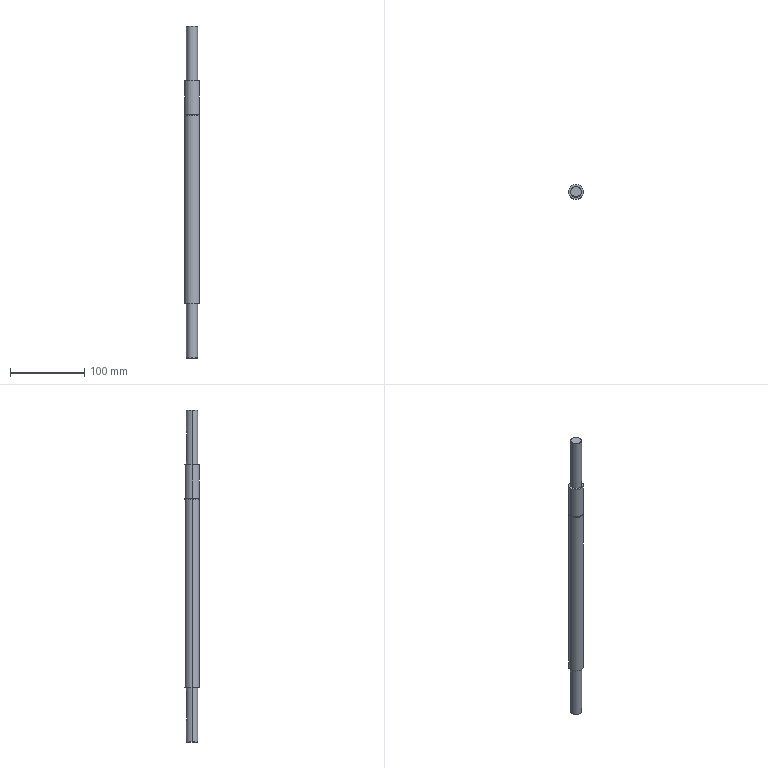Part | SolidWorks | features ICE 5, Chamfer 1, Cut 1, Extrusion 1 | 1 solid | 32 faces | box 20 x 20 x 448 mm | volume 119242 mm3 | cylinder 16 | plane 12 | cone 4 | commonest cylinder face diameters 5 x6 15 x4 20 x4 19 x2
STEP:
#1=CARTESIAN_POINT('',(10.,0.,300.));
#2=VERTEX_POINT('',#1);
#3=CARTESIAN_POINT('',(-10.,0.,300.));
#4=VERTEX_POINT('',#3);
#5=CARTESIAN_POINT('',(0.,0.,300.));
#6=DIRECTION('',(0.,0.,1.));
#7=DIRECTION('',(1.,0.,0.));
#8=AXIS2_PLACEMENT_3D('',#5,#6,#7);
#9=CIRCLE('',#8,10.);
#10=EDGE_CURVE('',#2,#4,#9,.T.);
#11=ORIENTED_EDGE('',*,*,#10,.F.);
#12=CARTESIAN_POINT('',(10.,0.,255.));
#13=VERTEX_POINT('',#12);
#14=CARTESIAN_POINT('',(10.,0.,300.));
#15=DIRECTION('',(0.,0.,-1.));
#16=VECTOR('',#15,1000.);
#17=LINE('',#14,#16);
#18=EDGE_CURVE('',#2,#13,#17,.T.);
#19=ORIENTED_EDGE('',*,*,#18,.T.);
#20=CARTESIAN_POINT('',(-10.,0.,255.));
#21=VERTEX_POINT('',#20);
#22=CARTESIAN_POINT('',(0.,0.,255.));
#23=DIRECTION('',(0.,0.,-1.));
#24=DIRECTION('',(0.,1.,0.));
#25=AXIS2_PLACEMENT_3D('',#22,#23,#24);
#26=CIRCLE('',#25,10.);
#27=EDGE_CURVE('',#21,#13,#26,.T.);
#28=ORIENTED_EDGE('',*,*,#27,.F.);
#29=CARTESIAN_POINT('',(-10.,0.,300.));
#30=DIRECTION('',(0.,0.,-1.));
#31=VECTOR('',#30,1000.);
#32=LINE('',#29,#31);
#33=EDGE_CURVE('',#4,#21,#32,.T.);
#34=ORIENTED_EDGE('',*,*,#33,.F.);
#35=EDGE_LOOP('',(#11,#19,#28,#34));
#36=FACE_OUTER_BOUND('',#35,.T.);
#37=CARTESIAN_POINT('',(0.,0.,300.));
#38=DIRECTION('',(0.,0.,-1.));
#39=DIRECTION('',(-1.,0.,0.));
#40=AXIS2_PLACEMENT_3D('',#37,#38,#39);
#41=CYLINDRICAL_SURFACE('',#40,10.);
#42=ADVANCED_FACE('',(#36),#41,.T.);
#43=CARTESIAN_POINT('',(2.5,7.071,343.));
#44=VERTEX_POINT('',#43);
#45=CARTESIAN_POINT('',(0.,7.5,345.5));
#46=VERTEX_POINT('',#45);
#47=CARTESIAN_POINT('',(2.5,7.071,343.));
#48=CARTESIAN_POINT('',(2.5,7.071,343.165));
#49=CARTESIAN_POINT('',(2.484,7.077,343.328));
#50=CARTESIAN_POINT('',(2.419,7.099,343.651));
#51=CARTESIAN_POINT('',(2.371,7.116,343.81));
#52=CARTESIAN_POINT('',(2.183,7.177,344.262));
#53=CARTESIAN_POINT('',(1.997,7.233,344.538));
#54=CARTESIAN_POINT('',(1.654,7.316,344.882));
#55=CARTESIAN_POINT('',(1.526,7.344,344.987));
#56=CARTESIAN_POINT('',(1.256,7.395,345.168));
#57=CARTESIAN_POINT('',(1.113,7.419,345.245));
#58=CARTESIAN_POINT('',(0.8106,7.458,345.371));
#59=CARTESIAN_POINT('',(0.6511,7.473,345.419));
#60=CARTESIAN_POINT('',(0.33,7.494,345.484));
#61=CARTESIAN_POINT('',(0.1664,7.5,345.5));
#62=CARTESIAN_POINT('',(0.,7.5,345.5));
#63=B_SPLINE_CURVE_WITH_KNOTS('',3,(#47,#48,#49,#50,#51,#52,#53,#54,#55,#56,#57,#58,#59,#60,#61,#62),.UNSPECIFIED.,.F.,.F.,(4,2,2,2,2,2,2,4),(0.01181,0.0123,0.01279,0.01378,0.01427,0.01476,0.01525,0.01574),.UNSPECIFIED.);
#64=EDGE_CURVE('',#44,#46,#63,.T.);
#65=ORIENTED_EDGE('',*,*,#64,.T.);
#66=CARTESIAN_POINT('',(-2.5,7.071,343.));
#67=VERTEX_POINT('',#66);
#68=CARTESIAN_POINT('',(0.,7.5,345.5));
#69=CARTESIAN_POINT('',(-0.1665,7.5,345.5));
#70=CARTESIAN_POINT('',(-0.33,7.494,345.484));
#71=CARTESIAN_POINT('',(-0.6513,7.473,345.419));
#72=CARTESIAN_POINT('',(-0.8108,7.458,345.371));
#73=CARTESIAN_POINT('',(-1.113,7.418,345.244));
#74=CARTESIAN_POINT('',(-1.256,7.395,345.167));
#75=CARTESIAN_POINT('',(-1.527,7.344,344.986));
#76=CARTESIAN_POINT('',(-1.655,7.316,344.881));
#77=CARTESIAN_POINT('',(-1.998,7.233,344.537));
#78=CARTESIAN_POINT('',(-2.183,7.176,344.26));
#79=CARTESIAN_POINT('',(-2.371,7.116,343.81));
#80=CARTESIAN_POINT('',(-2.419,7.099,343.651));
#81=CARTESIAN_POINT('',(-2.484,7.077,343.328));
#82=CARTESIAN_POINT('',(-2.5,7.071,343.164));
#83=CARTESIAN_POINT('',(-2.5,7.071,343.));
#84=B_SPLINE_CURVE_WITH_KNOTS('',3,(#68,#69,#70,#71,#72,#73,#74,#75,#76,#77,#78,#79,#80,#81,#82,#83),.UNSPECIFIED.,.F.,.F.,(4,2,2,2,2,2,2,4),(0.,0.0004922,0.0009844,0.001477,0.001969,0.002953,0.003445,0.003938),.UNSPECIFIED.);
#85=EDGE_CURVE('',#46,#67,#84,.T.);
#86=ORIENTED_EDGE('',*,*,#85,.T.);
#87=CARTESIAN_POINT('',(-2.5,7.071,308.));
#88=VERTEX_POINT('',#87);
#89=CARTESIAN_POINT('',(-2.5,7.071,374.));
#90=DIRECTION('',(0.,0.,-1.));
#91=VECTOR('',#90,1000.);
#92=LINE('',#89,#91);
#93=EDGE_CURVE('',#67,#88,#92,.T.);
#94=ORIENTED_EDGE('',*,*,#93,.T.);
#95=CARTESIAN_POINT('',(2.5,7.071,308.));
#96=VERTEX_POINT('',#95);
#97=CARTESIAN_POINT('',(-2.5,7.071,308.));
#98=CARTESIAN_POINT('',(-2.5,7.071,307.836));
#99=CARTESIAN_POINT('',(-2.483,7.077,307.669));
#100=CARTESIAN_POINT('',(-2.419,7.099,307.347));
#101=CARTESIAN_POINT('',(-2.371,7.116,307.191));
#102=CARTESIAN_POINT('',(-2.244,7.157,306.887));
#103=CARTESIAN_POINT('',(-2.167,7.181,306.743));
#104=CARTESIAN_POINT('',(-1.986,7.233,306.473));
#105=CARTESIAN_POINT('',(-1.882,7.261,306.346));
#106=CARTESIAN_POINT('',(-1.652,7.317,306.116));
#107=CARTESIAN_POINT('',(-1.527,7.344,306.014));
#108=CARTESIAN_POINT('',(-1.257,7.395,305.833));
#109=CARTESIAN_POINT('',(-1.11,7.419,305.754));
#110=CARTESIAN_POINT('',(-0.8093,7.458,305.629));
#111=CARTESIAN_POINT('',(-0.6533,7.473,305.581));
#112=CARTESIAN_POINT('',(-0.3296,7.495,305.516));
#113=CARTESIAN_POINT('',(-0.164,7.5,305.5));
#114=CARTESIAN_POINT('',(0.1639,7.5,305.5));
#115=CARTESIAN_POINT('',(0.329,7.495,305.516));
#116=CARTESIAN_POINT('',(0.6533,7.473,305.581));
#117=CARTESIAN_POINT('',(0.8096,7.458,305.629));
#118=CARTESIAN_POINT('',(1.111,7.419,305.755));
#119=CARTESIAN_POINT('',(1.257,7.395,305.833));
#120=CARTESIAN_POINT('',(1.527,7.344,306.014));
#121=CARTESIAN_POINT('',(1.653,7.317,306.117));
#122=CARTESIAN_POINT('',(1.999,7.233,306.463));
#123=CARTESIAN_POINT('',(2.182,7.177,306.736));
#124=CARTESIAN_POINT('',(2.371,7.116,307.192));
#125=CARTESIAN_POINT('',(2.419,7.099,307.348));
#126=CARTESIAN_POINT('',(2.483,7.077,307.669));
#127=CARTESIAN_POINT('',(2.5,7.071,307.835));
#128=CARTESIAN_POINT('',(2.5,7.071,308.));
#129=B_SPLINE_CURVE_WITH_KNOTS('',3,(#97,#98,#99,#100,#101,#102,#103,#104,#105,#106,#107,#108,#109,#110,#111,#112,#113,#114,#115,#116,#117,#118,#119,#120,#121,#122,#123,#124,#125,#126,#127,#128),.UNSPECIFIED.,.F.,.F.,(4,2,2,2,2,2,2,2,2,2,2,2,2,2,2,4),(0.003938,0.00443,0.004921,0.005413,0.005905,0.006397,0.006889,0.007381,0.007873,0.008365,0.008857,0.009349,0.00984,0.01082,0.01132,0.01181),.UNSPECIFIED.);
#130=EDGE_CURVE('',#88,#96,#129,.T.);
#131=ORIENTED_EDGE('',*,*,#130,.T.);
#132=CARTESIAN_POINT('',(2.5,7.071,374.));
#133=DIRECTION('',(0.,0.,1.));
#134=VECTOR('',#133,1000.);
#135=LINE('',#132,#134);
#136=EDGE_CURVE('',#96,#44,#135,.T.);
#137=ORIENTED_EDGE('',*,*,#136,.T.);
#138=EDGE_LOOP('',(#65,#86,#94,#131,#137));
#139=FACE_BOUND('',#138,.T.);
#140=CARTESIAN_POINT('',(-7.5,0.,373.5));
#141=VERTEX_POINT('',#140);
#142=CARTESIAN_POINT('',(7.5,0.,373.5));
#143=VERTEX_POINT('',#142);
#144=CARTESIAN_POINT('',(0.,0.,373.5));
#145=DIRECTION('',(0.,0.,-1.));
#146=DIRECTION('',(1.,0.,0.));
#147=AXIS2_PLACEMENT_3D('',#144,#145,#146);
#148=CIRCLE('',#147,7.5);
#149=EDGE_CURVE('',#141,#143,#148,.T.);
#150=ORIENTED_EDGE('',*,*,#149,.T.);
#151=CARTESIAN_POINT('',(7.5,0.,300.));
#152=VERTEX_POINT('',#151);
#153=CARTESIAN_POINT('',(7.5,0.,374.));
#154=DIRECTION('',(0.,0.,-1.));
#155=VECTOR('',#154,1000.);
#156=LINE('',#153,#155);
#157=EDGE_CURVE('',#143,#152,#156,.T.);
#158=ORIENTED_EDGE('',*,*,#157,.T.);
#159=CARTESIAN_POINT('',(-7.5,0.,300.));
#160=VERTEX_POINT('',#159);
#161=CARTESIAN_POINT('',(0.,0.,300.));
#162=DIRECTION('',(0.,0.,1.));
#163=DIRECTION('',(1.,0.,0.));
#164=AXIS2_PLACEMENT_3D('',#161,#162,#163);
#165=CIRCLE('',#164,7.5);
#166=EDGE_CURVE('',#152,#160,#165,.T.);
#167=ORIENTED_EDGE('',*,*,#166,.T.);
#168=CARTESIAN_POINT('',(-7.5,0.,374.));
#169=DIRECTION('',(0.,0.,-1.));
#170=VECTOR('',#169,1000.);
#171=LINE('',#168,#170);
#172=EDGE_CURVE('',#141,#160,#171,.T.);
#173=ORIENTED_EDGE('',*,*,#172,.F.);
#174=EDGE_LOOP('',(#150,#158,#167,#173));
#175=FACE_OUTER_BOUND('',#174,.T.);
#176=CARTESIAN_POINT('',(0.,0.,374.));
#177=DIRECTION('',(0.,0.,-1.));
#178=DIRECTION('',(-1.,0.,0.));
#179=AXIS2_PLACEMENT_3D('',#176,#177,#178);
#180=CYLINDRICAL_SURFACE('',#179,7.5);
#181=ADVANCED_FACE('',(#139,#175),#180,.T.);
#182=CARTESIAN_POINT('',(7.,0.,374.));
#183=VERTEX_POINT('',#182);
#184=CARTESIAN_POINT('',(-7.,0.,374.));
#185=VERTEX_POINT('',#184);
#186=CARTESIAN_POINT('',(0.,0.,374.));
#187=DIRECTION('',(0.,0.,1.));
#188=DIRECTION('',(1.,0.,0.));
#189=AXIS2_PLACEMENT_3D('',#186,#187,#188);
#190=CIRCLE('',#189,7.);
#191=EDGE_CURVE('',#183,#185,#190,.T.);
#192=ORIENTED_EDGE('',*,*,#191,.F.);
#193=CARTESIAN_POINT('',(7.,0.,374.));
#194=DIRECTION('',(0.7071,0.,-0.7071));
#195=VECTOR('',#194,1000.);
#196=LINE('',#193,#195);
#197=EDGE_CURVE('',#183,#143,#196,.T.);
#198=ORIENTED_EDGE('',*,*,#197,.T.);
#199=ORIENTED_EDGE('',*,*,#149,.F.);
#200=CARTESIAN_POINT('',(-7.,0.,374.));
#201=DIRECTION('',(-0.7071,0.,-0.7071));
#202=VECTOR('',#201,1000.);
#203=LINE('',#200,#202);
#204=EDGE_CURVE('',#185,#141,#203,.T.);
#205=ORIENTED_EDGE('',*,*,#204,.F.);
#206=EDGE_LOOP('',(#192,#198,#199,#205));
#207=FACE_OUTER_BOUND('',#206,.T.);
#208=CARTESIAN_POINT('',(0.,0.,374.));
#209=DIRECTION('',(0.,0.,-1.));
#210=DIRECTION('',(-1.,0.,0.));
#211=AXIS2_PLACEMENT_3D('',#208,#209,#210);
#212=CONICAL_SURFACE('',#211,7.,0.7854);
#213=ADVANCED_FACE('',(#207),#212,.T.);
#214=CARTESIAN_POINT('',(0.,4.5,345.5));
#215=VERTEX_POINT('',#214);
#216=CARTESIAN_POINT('',(2.5,4.5,343.));
#217=VERTEX_POINT('',#216);
#218=CARTESIAN_POINT('',(0.,4.5,343.));
#219=DIRECTION('',(0.,1.,0.));
#220=DIRECTION('',(0.,0.,1.));
#221=AXIS2_PLACEMENT_3D('',#218,#219,#220);
#222=CIRCLE('',#221,2.5);
#223=EDGE_CURVE('',#215,#217,#222,.T.);
#224=ORIENTED_EDGE('',*,*,#223,.F.);
#225=CARTESIAN_POINT('',(0.,4.5,345.5));
#226=DIRECTION('',(0.,1.,0.));
#227=VECTOR('',#226,1000.);
#228=LINE('',#225,#227);
#229=EDGE_CURVE('',#215,#46,#228,.T.);
#230=ORIENTED_EDGE('',*,*,#229,.T.);
#231=ORIENTED_EDGE('',*,*,#64,.F.);
#232=CARTESIAN_POINT('',(2.5,4.5,343.));
#233=DIRECTION('',(0.,1.,0.));
#234=VECTOR('',#233,1000.);
#235=LINE('',#232,#234);
#236=EDGE_CURVE('',#217,#44,#235,.T.);
#237=ORIENTED_EDGE('',*,*,#236,.F.);
#238=EDGE_LOOP('',(#224,#230,#231,#237));
#239=FACE_OUTER_BOUND('',#238,.T.);
#240=CARTESIAN_POINT('',(0.,4.5,343.));
#241=DIRECTION('',(0.,1.,0.));
#242=DIRECTION('',(0.,0.,1.));
#243=AXIS2_PLACEMENT_3D('',#240,#241,#242);
#244=CYLINDRICAL_SURFACE('',#243,2.5);
#245=ADVANCED_FACE('',(#239),#244,.F.);
#246=CARTESIAN_POINT('',(0.,9.5,253.9));
#247=VERTEX_POINT('',#246);
#248=CARTESIAN_POINT('',(0.,-9.5,253.9));
#249=VERTEX_POINT('',#248);
#250=CARTESIAN_POINT('',(0.,0.,253.9));
#251=DIRECTION('',(0.,0.,-1.));
#252=DIRECTION('',(0.,1.,0.));
#253=AXIS2_PLACEMENT_3D('',#250,#251,#252);
#254=CIRCLE('',#253,9.5);
#255=EDGE_CURVE('',#247,#249,#254,.T.);
#256=ORIENTED_EDGE('',*,*,#255,.F.);
#257=CARTESIAN_POINT('',(0.,9.5,255.));
#258=VERTEX_POINT('',#257);
#259=CARTESIAN_POINT('',(0.,9.5,253.9));
#260=DIRECTION('',(0.,0.,1.));
#261=VECTOR('',#260,1000.);
#262=LINE('',#259,#261);
#263=EDGE_CURVE('',#247,#258,#262,.T.);
#264=ORIENTED_EDGE('',*,*,#263,.T.);
#265=CARTESIAN_POINT('',(0.,-9.5,255.));
#266=VERTEX_POINT('',#265);
#267=CARTESIAN_POINT('',(0.,0.,255.));
#268=DIRECTION('',(0.,0.,-1.));
#269=DIRECTION('',(0.,1.,0.));
#270=AXIS2_PLACEMENT_3D('',#267,#268,#269);
#271=CIRCLE('',#270,9.5);
#272=EDGE_CURVE('',#258,#266,#271,.T.);
#273=ORIENTED_EDGE('',*,*,#272,.T.);
#274=CARTESIAN_POINT('',(0.,-9.5,253.9));
#275=DIRECTION('',(0.,0.,1.));
#276=VECTOR('',#275,1000.);
#277=LINE('',#274,#276);
#278=EDGE_CURVE('',#249,#266,#277,.T.);
#279=ORIENTED_EDGE('',*,*,#278,.F.);
#280=EDGE_LOOP('',(#256,#264,#273,#279));
#281=FACE_OUTER_BOUND('',#280,.T.);
#282=CARTESIAN_POINT('',(0.,0.,253.9));
#283=DIRECTION('',(0.,0.,1.));
#284=DIRECTION('',(0.,-1.,0.));
#285=AXIS2_PLACEMENT_3D('',#282,#283,#284);
#286=CYLINDRICAL_SURFACE('',#285,9.5);
#287=ADVANCED_FACE('',(#281),#286,.T.);
#288=CARTESIAN_POINT('',(-7.,0.,-74.));
#289=VERTEX_POINT('',#288);
#290=CARTESIAN_POINT('',(7.,0.,-74.));
#291=VERTEX_POINT('',#290);
#292=CARTESIAN_POINT('',(0.,0.,-74.));
#293=DIRECTION('',(0.,0.,-1.));
#294=DIRECTION('',(-1.,0.,0.));
#295=AXIS2_PLACEMENT_3D('',#292,#293,#294);
#296=CIRCLE('',#295,7.);
#297=EDGE_CURVE('',#289,#291,#296,.T.);
#298=ORIENTED_EDGE('',*,*,#297,.F.);
#299=CARTESIAN_POINT('',(-7.5,0.,-73.5));
#300=VERTEX_POINT('',#299);
#301=CARTESIAN_POINT('',(-7.,0.,-74.));
#302=DIRECTION('',(-0.7071,0.,0.7071));
#303=VECTOR('',#302,1000.);
#304=LINE('',#301,#303);
#305=EDGE_CURVE('',#289,#300,#304,.T.);
#306=ORIENTED_EDGE('',*,*,#305,.T.);
#307=CARTESIAN_POINT('',(7.5,0.,-73.5));
#308=VERTEX_POINT('',#307);
#309=CARTESIAN_POINT('',(0.,0.,-73.5));
#310=DIRECTION('',(0.,0.,1.));
#311=DIRECTION('',(-1.,0.,0.));
#312=AXIS2_PLACEMENT_3D('',#309,#310,#311);
#313=CIRCLE('',#312,7.5);
#314=EDGE_CURVE('',#308,#300,#313,.T.);
#315=ORIENTED_EDGE('',*,*,#314,.F.);
#316=CARTESIAN_POINT('',(7.,0.,-74.));
#317=DIRECTION('',(0.7071,0.,0.7071));
#318=VECTOR('',#317,1000.);
#319=LINE('',#316,#318);
#320=EDGE_CURVE('',#291,#308,#319,.T.);
#321=ORIENTED_EDGE('',*,*,#320,.F.);
#322=EDGE_LOOP('',(#298,#306,#315,#321));
#323=FACE_OUTER_BOUND('',#322,.T.);
#324=CARTESIAN_POINT('',(0.,0.,-74.));
#325=DIRECTION('',(0.,0.,1.));
#326=DIRECTION('',(1.,0.,0.));
#327=AXIS2_PLACEMENT_3D('',#324,#325,#326);
#328=CONICAL_SURFACE('',#327,7.,0.7854);
#329=ADVANCED_FACE('',(#323),#328,.T.);
#330=CARTESIAN_POINT('',(0.,4.5,-5.5));
#331=VERTEX_POINT('',#330);
#332=CARTESIAN_POINT('',(2.5,4.5,-8.));
#333=VERTEX_POINT('',#332);
#334=CARTESIAN_POINT('',(0.,4.5,-8.));
#335=DIRECTION('',(0.,1.,0.));
#336=DIRECTION('',(0.,0.,1.));
#337=AXIS2_PLACEMENT_3D('',#334,#335,#336);
#338=CIRCLE('',#337,2.5);
#339=EDGE_CURVE('',#331,#333,#338,.T.);
#340=ORIENTED_EDGE('',*,*,#339,.F.);
#341=CARTESIAN_POINT('',(0.,7.5,-5.5));
#342=VERTEX_POINT('',#341);
#343=CARTESIAN_POINT('',(0.,4.5,-5.5));
#344=DIRECTION('',(0.,1.,0.));
#345=VECTOR('',#344,1000.);
#346=LINE('',#343,#345);
#347=EDGE_CURVE('',#331,#342,#346,.T.);
#348=ORIENTED_EDGE('',*,*,#347,.T.);
#349=CARTESIAN_POINT('',(2.5,7.071,-8.));
#350=VERTEX_POINT('',#349);
#351=CARTESIAN_POINT('',(2.5,7.071,-8.));
#352=CARTESIAN_POINT('',(2.5,7.071,-7.835));
#353=CARTESIAN_POINT('',(2.484,7.077,-7.672));
#354=CARTESIAN_POINT('',(2.419,7.099,-7.349));
#355=CARTESIAN_POINT('',(2.371,7.116,-7.19));
#356=CARTESIAN_POINT('',(2.183,7.177,-6.738));
#357=CARTESIAN_POINT('',(1.997,7.233,-6.462));
#358=CARTESIAN_POINT('',(1.654,7.316,-6.118));
#359=CARTESIAN_POINT('',(1.526,7.344,-6.013));
#360=CARTESIAN_POINT('',(1.256,7.395,-5.832));
#361=CARTESIAN_POINT('',(1.113,7.419,-5.755));
#362=CARTESIAN_POINT('',(0.8106,7.458,-5.629));
#363=CARTESIAN_POINT('',(0.6511,7.473,-5.581));
#364=CARTESIAN_POINT('',(0.33,7.494,-5.516));
#365=CARTESIAN_POINT('',(0.1664,7.5,-5.5));
#366=CARTESIAN_POINT('',(0.,7.5,-5.5));
#367=B_SPLINE_CURVE_WITH_KNOTS('',3,(#351,#352,#353,#354,#355,#356,#357,#358,#359,#360,#361,#362,#363,#364,#365,#366),.UNSPECIFIED.,.F.,.F.,(4,2,2,2,2,2,2,4),(0.01181,0.0123,0.01279,0.01378,0.01427,0.01476,0.01525,0.01574),.UNSPECIFIED.);
#368=EDGE_CURVE('',#350,#342,#367,.T.);
#369=ORIENTED_EDGE('',*,*,#368,.F.);
#370=CARTESIAN_POINT('',(2.5,4.5,-8.));
#371=DIRECTION('',(0.,1.,0.));
#372=VECTOR('',#371,1000.);
#373=LINE('',#370,#372);
#374=EDGE_CURVE('',#333,#350,#373,.T.);
#375=ORIENTED_EDGE('',*,*,#374,.F.);
#376=EDGE_LOOP('',(#340,#348,#369,#375));
#377=FACE_OUTER_BOUND('',#376,.T.);
#378=CARTESIAN_POINT('',(0.,4.5,-8.));
#379=DIRECTION('',(0.,1.,0.));
#380=DIRECTION('',(0.,0.,1.));
#381=AXIS2_PLACEMENT_3D('',#378,#379,#380);
#382=CYLINDRICAL_SURFACE('',#381,2.5);
#383=ADVANCED_FACE('',(#377),#382,.F.);
#384=ORIENTED_EDGE('',*,*,#368,.T.);
#385=CARTESIAN_POINT('',(-2.5,7.071,-8.));
#386=VERTEX_POINT('',#385);
#387=CARTESIAN_POINT('',(0.,7.5,-5.5));
#388=CARTESIAN_POINT('',(-0.1665,7.5,-5.5));
#389=CARTESIAN_POINT('',(-0.33,7.494,-5.516));
#390=CARTESIAN_POINT('',(-0.6513,7.473,-5.581));
#391=CARTESIAN_POINT('',(-0.8108,7.458,-5.629));
#392=CARTESIAN_POINT('',(-1.113,7.418,-5.756));
#393=CARTESIAN_POINT('',(-1.256,7.395,-5.833));
#394=CARTESIAN_POINT('',(-1.527,7.344,-6.014));
#395=CARTESIAN_POINT('',(-1.655,7.316,-6.119));
#396=CARTESIAN_POINT('',(-1.998,7.233,-6.463));
#397=CARTESIAN_POINT('',(-2.183,7.176,-6.74));
#398=CARTESIAN_POINT('',(-2.371,7.116,-7.19));
#399=CARTESIAN_POINT('',(-2.419,7.099,-7.349));
#400=CARTESIAN_POINT('',(-2.484,7.077,-7.672));
#401=CARTESIAN_POINT('',(-2.5,7.071,-7.836));
#402=CARTESIAN_POINT('',(-2.5,7.071,-8.));
#403=B_SPLINE_CURVE_WITH_KNOTS('',3,(#387,#388,#389,#390,#391,#392,#393,#394,#395,#396,#397,#398,#399,#400,#401,#402),.UNSPECIFIED.,.F.,.F.,(4,2,2,2,2,2,2,4),(0.,0.0004922,0.0009844,0.001477,0.001969,0.002953,0.003445,0.003938),.UNSPECIFIED.);
#404=EDGE_CURVE('',#342,#386,#403,.T.);
#405=ORIENTED_EDGE('',*,*,#404,.T.);
#406=CARTESIAN_POINT('',(-2.5,7.071,-43.));
#407=VERTEX_POINT('',#406);
#408=CARTESIAN_POINT('',(-2.5,7.071,-74.));
#409=DIRECTION('',(0.,0.,-1.));
#410=VECTOR('',#409,1000.);
#411=LINE('',#408,#410);
#412=EDGE_CURVE('',#386,#407,#411,.T.);
#413=ORIENTED_EDGE('',*,*,#412,.T.);
#414=CARTESIAN_POINT('',(2.5,7.071,-43.));
#415=VERTEX_POINT('',#414);
#416=CARTESIAN_POINT('',(-2.5,7.071,-43.));
#417=CARTESIAN_POINT('',(-2.5,7.071,-43.164));
#418=CARTESIAN_POINT('',(-2.483,7.077,-43.331));
#419=CARTESIAN_POINT('',(-2.419,7.099,-43.653));
#420=CARTESIAN_POINT('',(-2.371,7.116,-43.809));
#421=CARTESIAN_POINT('',(-2.244,7.157,-44.113));
#422=CARTESIAN_POINT('',(-2.167,7.181,-44.257));
#423=CARTESIAN_POINT('',(-1.986,7.233,-44.527));
#424=CARTESIAN_POINT('',(-1.882,7.261,-44.654));
#425=CARTESIAN_POINT('',(-1.652,7.317,-44.884));
#426=CARTESIAN_POINT('',(-1.527,7.344,-44.986));
#427=CARTESIAN_POINT('',(-1.257,7.395,-45.167));
#428=CARTESIAN_POINT('',(-1.11,7.419,-45.246));
#429=CARTESIAN_POINT('',(-0.8093,7.458,-45.371));
#430=CARTESIAN_POINT('',(-0.6533,7.473,-45.419));
#431=CARTESIAN_POINT('',(-0.3296,7.495,-45.484));
#432=CARTESIAN_POINT('',(-0.164,7.5,-45.5));
#433=CARTESIAN_POINT('',(0.1639,7.5,-45.5));
#434=CARTESIAN_POINT('',(0.329,7.495,-45.484));
#435=CARTESIAN_POINT('',(0.6533,7.473,-45.419));
#436=CARTESIAN_POINT('',(0.8096,7.458,-45.371));
#437=CARTESIAN_POINT('',(1.111,7.419,-45.245));
#438=CARTESIAN_POINT('',(1.257,7.395,-45.167));
#439=CARTESIAN_POINT('',(1.527,7.344,-44.986));
#440=CARTESIAN_POINT('',(1.653,7.317,-44.883));
#441=CARTESIAN_POINT('',(1.999,7.233,-44.537));
#442=CARTESIAN_POINT('',(2.182,7.177,-44.264));
#443=CARTESIAN_POINT('',(2.371,7.116,-43.808));
#444=CARTESIAN_POINT('',(2.419,7.099,-43.652));
#445=CARTESIAN_POINT('',(2.483,7.077,-43.331));
#446=CARTESIAN_POINT('',(2.5,7.071,-43.165));
#447=CARTESIAN_POINT('',(2.5,7.071,-43.));
#448=B_SPLINE_CURVE_WITH_KNOTS('',3,(#416,#417,#418,#419,#420,#421,#422,#423,#424,#425,#426,#427,#428,#429,#430,#431,#432,#433,#434,#435,#436,#437,#438,#439,#440,#441,#442,#443,#444,#445,#446,#447),.UNSPECIFIED.,.F.,.F.,(4,2,2,2,2,2,2,2,2,2,2,2,2,2,2,4),(0.003938,0.00443,0.004921,0.005413,0.005905,0.006397,0.006889,0.007381,0.007873,0.008365,0.008857,0.009349,0.00984,0.01082,0.01132,0.01181),.UNSPECIFIED.);
#449=EDGE_CURVE('',#407,#415,#448,.T.);
#450=ORIENTED_EDGE('',*,*,#449,.T.);
#451=CARTESIAN_POINT('',(2.5,7.071,-74.));
#452=DIRECTION('',(0.,0.,1.));
#453=VECTOR('',#452,1000.);
#454=LINE('',#451,#453);
#455=EDGE_CURVE('',#415,#350,#454,.T.);
#456=ORIENTED_EDGE('',*,*,#455,.T.);
#457=EDGE_LOOP('',(#384,#405,#413,#450,#456));
#458=FACE_BOUND('',#457,.T.);
#459=ORIENTED_EDGE('',*,*,#314,.T.);
#460=CARTESIAN_POINT('',(-7.5,0.,0.));
#461=VERTEX_POINT('',#460);
#462=CARTESIAN_POINT('',(-7.5,0.,-74.));
#463=DIRECTION('',(0.,0.,1.));
#464=VECTOR('',#463,1000.);
#465=LINE('',#462,#464);
#466=EDGE_CURVE('',#300,#461,#465,.T.);
#467=ORIENTED_EDGE('',*,*,#466,.T.);
#468=CARTESIAN_POINT('',(7.5,0.,0.));
#469=VERTEX_POINT('',#468);
#470=CARTESIAN_POINT('',(0.,0.,0.));
#471=DIRECTION('',(0.,0.,-1.));
#472=DIRECTION('',(1.,0.,0.));
#473=AXIS2_PLACEMENT_3D('',#470,#471,#472);
#474=CIRCLE('',#473,7.5);
#475=EDGE_CURVE('',#461,#469,#474,.T.);
#476=ORIENTED_EDGE('',*,*,#475,.T.);
#477=CARTESIAN_POINT('',(7.5,0.,-74.));
#478=DIRECTION('',(0.,0.,1.));
#479=VECTOR('',#478,1000.);
#480=LINE('',#477,#479);
#481=EDGE_CURVE('',#308,#469,#480,.T.);
#482=ORIENTED_EDGE('',*,*,#481,.F.);
#483=EDGE_LOOP('',(#459,#467,#476,#482));
#484=FACE_OUTER_BOUND('',#483,.T.);
#485=CARTESIAN_POINT('',(0.,0.,-74.));
#486=DIRECTION('',(0.,0.,1.));
#487=DIRECTION('',(1.,0.,0.));
#488=AXIS2_PLACEMENT_3D('',#485,#486,#487);
#489=CYLINDRICAL_SURFACE('',#488,7.5);
#490=ADVANCED_FACE('',(#458,#484),#489,.T.);
#491=CARTESIAN_POINT('',(-10.,0.,253.9));
#492=VERTEX_POINT('',#491);
#493=CARTESIAN_POINT('',(10.,0.,253.9));
#494=VERTEX_POINT('',#493);
#495=CARTESIAN_POINT('',(0.,0.,253.9));
#496=DIRECTION('',(0.,0.,-1.));
#497=DIRECTION('',(0.,1.,0.));
#498=AXIS2_PLACEMENT_3D('',#495,#496,#497);
#499=CIRCLE('',#498,10.);
#500=EDGE_CURVE('',#492,#494,#499,.T.);
#501=ORIENTED_EDGE('',*,*,#500,.T.);
#502=CARTESIAN_POINT('',(10.,0.,0.));
#503=VERTEX_POINT('',#502);
#504=CARTESIAN_POINT('',(10.,0.,300.));
#505=DIRECTION('',(0.,0.,-1.));
#506=VECTOR('',#505,1000.);
#507=LINE('',#504,#506);
#508=EDGE_CURVE('',#494,#503,#507,.T.);
#509=ORIENTED_EDGE('',*,*,#508,.T.);
#510=CARTESIAN_POINT('',(-10.,0.,0.));
#511=VERTEX_POINT('',#510);
#512=CARTESIAN_POINT('',(0.,0.,0.));
#513=DIRECTION('',(0.,0.,1.));
#514=DIRECTION('',(1.,0.,0.));
#515=AXIS2_PLACEMENT_3D('',#512,#513,#514);
#516=CIRCLE('',#515,10.);
#517=EDGE_CURVE('',#503,#511,#516,.T.);
#518=ORIENTED_EDGE('',*,*,#517,.T.);
#519=CARTESIAN_POINT('',(-10.,0.,300.));
#520=DIRECTION('',(0.,0.,-1.));
#521=VECTOR('',#520,1000.);
#522=LINE('',#519,#521);
#523=EDGE_CURVE('',#492,#511,#522,.T.);
#524=ORIENTED_EDGE('',*,*,#523,.F.);
#525=EDGE_LOOP('',(#501,#509,#518,#524));
#526=FACE_OUTER_BOUND('',#525,.T.);
#527=CARTESIAN_POINT('',(0.,0.,300.));
#528=DIRECTION('',(0.,0.,-1.));
#529=DIRECTION('',(-1.,0.,0.));
#530=AXIS2_PLACEMENT_3D('',#527,#528,#529);
#531=CYLINDRICAL_SURFACE('',#530,10.);
#532=ADVANCED_FACE('',(#526),#531,.T.);
#533=CARTESIAN_POINT('',(0.,0.,0.));
#534=DIRECTION('',(0.,0.,1.));
#535=DIRECTION('',(1.,0.,0.));
#536=AXIS2_PLACEMENT_3D('',#533,#534,#535);
#537=CIRCLE('',#536,10.);
#538=EDGE_CURVE('',#511,#503,#537,.T.);
#539=ORIENTED_EDGE('',*,*,#538,.F.);
#540=ORIENTED_EDGE('',*,*,#517,.F.);
#541=EDGE_LOOP('',(#539,#540));
#542=FACE_OUTER_BOUND('',#541,.T.);
#543=CARTESIAN_POINT('',(0.,0.,0.));
#544=DIRECTION('',(0.,0.,-1.));
#545=DIRECTION('',(1.,0.,0.));
#546=AXIS2_PLACEMENT_3D('',#543,#544,#545);
#547=CIRCLE('',#546,7.5);
#548=EDGE_CURVE('',#469,#461,#547,.T.);
#549=ORIENTED_EDGE('',*,*,#548,.F.);
#550=ORIENTED_EDGE('',*,*,#475,.F.);
#551=EDGE_LOOP('',(#549,#550));
#552=FACE_BOUND('',#551,.T.);
#553=CARTESIAN_POINT('',(0.,0.,0.));
#554=DIRECTION('',(0.,0.,1.));
#555=DIRECTION('',(1.,0.,0.));
#556=AXIS2_PLACEMENT_3D('',#553,#554,#555);
#557=PLANE('',#556);
#558=ADVANCED_FACE('',(#542,#552),#557,.F.);
#559=ORIENTED_EDGE('',*,*,#508,.F.);
#560=CARTESIAN_POINT('',(0.,0.,253.9));
#561=DIRECTION('',(0.,0.,-1.));
#562=DIRECTION('',(0.,1.,0.));
#563=AXIS2_PLACEMENT_3D('',#560,#561,#562);
#564=CIRCLE('',#563,10.);
#565=EDGE_CURVE('',#494,#492,#564,.T.);
#566=ORIENTED_EDGE('',*,*,#565,.T.);
#567=ORIENTED_EDGE('',*,*,#523,.T.);
#568=ORIENTED_EDGE('',*,*,#538,.T.);
#569=EDGE_LOOP('',(#559,#566,#567,#568));
#570=FACE_OUTER_BOUND('',#569,.T.);
#571=CARTESIAN_POINT('',(0.,0.,300.));
#572=DIRECTION('',(0.,0.,-1.));
#573=DIRECTION('',(-1.,0.,0.));
#574=AXIS2_PLACEMENT_3D('',#571,#572,#573);
#575=CYLINDRICAL_SURFACE('',#574,10.);
#576=ADVANCED_FACE('',(#570),#575,.T.);
#577=ORIENTED_EDGE('',*,*,#466,.F.);
#578=CARTESIAN_POINT('',(0.,0.,-73.5));
#579=DIRECTION('',(0.,0.,1.));
#580=DIRECTION('',(-1.,0.,0.));
#581=AXIS2_PLACEMENT_3D('',#578,#579,#580);
#582=CIRCLE('',#581,7.5);
#583=EDGE_CURVE('',#300,#308,#582,.T.);
#584=ORIENTED_EDGE('',*,*,#583,.T.);
#585=ORIENTED_EDGE('',*,*,#481,.T.);
#586=ORIENTED_EDGE('',*,*,#548,.T.);
#587=EDGE_LOOP('',(#577,#584,#585,#586));
#588=FACE_OUTER_BOUND('',#587,.T.);
#589=CARTESIAN_POINT('',(0.,0.,-74.));
#590=DIRECTION('',(0.,0.,1.));
#591=DIRECTION('',(1.,0.,0.));
#592=AXIS2_PLACEMENT_3D('',#589,#590,#591);
#593=CYLINDRICAL_SURFACE('',#592,7.5);
#594=ADVANCED_FACE('',(#588),#593,.T.);
#595=CARTESIAN_POINT('',(0.,0.,-74.));
#596=DIRECTION('',(0.,0.,-1.));
#597=DIRECTION('',(-1.,0.,0.));
#598=AXIS2_PLACEMENT_3D('',#595,#596,#597);
#599=CIRCLE('',#598,7.);
#600=EDGE_CURVE('',#291,#289,#599,.T.);
#601=ORIENTED_EDGE('',*,*,#600,.T.);
#602=ORIENTED_EDGE('',*,*,#297,.T.);
#603=EDGE_LOOP('',(#601,#602));
#604=FACE_OUTER_BOUND('',#603,.T.);
#605=CARTESIAN_POINT('',(0.,0.,-74.));
#606=DIRECTION('',(0.,0.,-1.));
#607=DIRECTION('',(-1.,0.,0.));
#608=AXIS2_PLACEMENT_3D('',#605,#606,#607);
#609=PLANE('',#608);
#610=ADVANCED_FACE('',(#604),#609,.T.);
#611=ORIENTED_EDGE('',*,*,#347,.F.);
#612=CARTESIAN_POINT('',(-2.5,4.5,-8.));
#613=VERTEX_POINT('',#612);
#614=CARTESIAN_POINT('',(0.,4.5,-8.));
#615=DIRECTION('',(0.,1.,0.));
#616=DIRECTION('',(0.,0.,1.));
#617=AXIS2_PLACEMENT_3D('',#614,#615,#616);
#618=CIRCLE('',#617,2.5);
#619=EDGE_CURVE('',#613,#331,#618,.T.);
#620=ORIENTED_EDGE('',*,*,#619,.F.);
#621=CARTESIAN_POINT('',(-2.5,4.5,-8.));
#622=DIRECTION('',(0.,1.,0.));
#623=VECTOR('',#622,1000.);
#624=LINE('',#621,#623);
#625=EDGE_CURVE('',#613,#386,#624,.T.);
#626=ORIENTED_EDGE('',*,*,#625,.T.);
#627=ORIENTED_EDGE('',*,*,#404,.F.);
#628=EDGE_LOOP('',(#611,#620,#626,#627));
#629=FACE_OUTER_BOUND('',#628,.T.);
#630=CARTESIAN_POINT('',(0.,4.5,-8.));
#631=DIRECTION('',(0.,1.,0.));
#632=DIRECTION('',(0.,0.,1.));
#633=AXIS2_PLACEMENT_3D('',#630,#631,#632);
#634=CYLINDRICAL_SURFACE('',#633,2.5);
#635=ADVANCED_FACE('',(#629),#634,.F.);
#636=ORIENTED_EDGE('',*,*,#625,.F.);
#637=CARTESIAN_POINT('',(-2.5,4.5,-43.));
#638=VERTEX_POINT('',#637);
#639=CARTESIAN_POINT('',(-2.5,4.5,-8.));
#640=DIRECTION('',(0.,0.,1.));
#641=VECTOR('',#640,1000.);
#642=LINE('',#639,#641);
#643=EDGE_CURVE('',#638,#613,#642,.T.);
#644=ORIENTED_EDGE('',*,*,#643,.F.);
#645=CARTESIAN_POINT('',(-2.5,4.5,-43.));
#646=DIRECTION('',(0.,1.,0.));
#647=VECTOR('',#646,1000.);
#648=LINE('',#645,#647);
#649=EDGE_CURVE('',#638,#407,#648,.T.);
#650=ORIENTED_EDGE('',*,*,#649,.T.);
#651=ORIENTED_EDGE('',*,*,#412,.F.);
#652=EDGE_LOOP('',(#636,#644,#650,#651));
#653=FACE_OUTER_BOUND('',#652,.T.);
#654=CARTESIAN_POINT('',(-2.5,4.5,-8.));
#655=DIRECTION('',(-1.,0.,0.));
#656=DIRECTION('',(0.,0.,1.));
#657=AXIS2_PLACEMENT_3D('',#654,#655,#656);
#658=PLANE('',#657);
#659=ADVANCED_FACE('',(#653),#658,.F.);
#660=ORIENTED_EDGE('',*,*,#649,.F.);
#661=CARTESIAN_POINT('',(2.5,4.5,-43.));
#662=VERTEX_POINT('',#661);
#663=CARTESIAN_POINT('',(0.,4.5,-43.));
#664=DIRECTION('',(0.,1.,0.));
#665=DIRECTION('',(0.,0.,1.));
#666=AXIS2_PLACEMENT_3D('',#663,#664,#665);
#667=CIRCLE('',#666,2.5);
#668=EDGE_CURVE('',#662,#638,#667,.T.);
#669=ORIENTED_EDGE('',*,*,#668,.F.);
#670=CARTESIAN_POINT('',(2.5,4.5,-43.));
#671=DIRECTION('',(0.,1.,0.));
#672=VECTOR('',#671,1000.);
#673=LINE('',#670,#672);
#674=EDGE_CURVE('',#662,#415,#673,.T.);
#675=ORIENTED_EDGE('',*,*,#674,.T.);
#676=ORIENTED_EDGE('',*,*,#449,.F.);
#677=EDGE_LOOP('',(#660,#669,#675,#676));
#678=FACE_OUTER_BOUND('',#677,.T.);
#679=CARTESIAN_POINT('',(0.,4.5,-43.));
#680=DIRECTION('',(0.,1.,0.));
#681=DIRECTION('',(0.,0.,1.));
#682=AXIS2_PLACEMENT_3D('',#679,#680,#681);
#683=CYLINDRICAL_SURFACE('',#682,2.5);
#684=ADVANCED_FACE('',(#678),#683,.F.);
#685=ORIENTED_EDGE('',*,*,#674,.F.);
#686=CARTESIAN_POINT('',(2.5,4.5,-8.));
#687=DIRECTION('',(0.,0.,-1.));
#688=VECTOR('',#687,1000.);
#689=LINE('',#686,#688);
#690=EDGE_CURVE('',#333,#662,#689,.T.);
#691=ORIENTED_EDGE('',*,*,#690,.F.);
#692=ORIENTED_EDGE('',*,*,#374,.T.);
#693=ORIENTED_EDGE('',*,*,#455,.F.);
#694=EDGE_LOOP('',(#685,#691,#692,#693));
#695=FACE_OUTER_BOUND('',#694,.T.);
#696=CARTESIAN_POINT('',(2.5,4.5,-8.));
#697=DIRECTION('',(1.,0.,0.));
#698=DIRECTION('',(0.,0.,-1.));
#699=AXIS2_PLACEMENT_3D('',#696,#697,#698);
#700=PLANE('',#699);
#701=ADVANCED_FACE('',(#695),#700,.F.);
#702=ORIENTED_EDGE('',*,*,#619,.T.);
#703=ORIENTED_EDGE('',*,*,#339,.T.);
#704=ORIENTED_EDGE('',*,*,#690,.T.);
#705=ORIENTED_EDGE('',*,*,#668,.T.);
#706=ORIENTED_EDGE('',*,*,#643,.T.);
#707=EDGE_LOOP('',(#702,#703,#704,#705,#706));
#708=FACE_OUTER_BOUND('',#707,.T.);
#709=CARTESIAN_POINT('',(0.,4.5,-8.));
#710=DIRECTION('',(0.,1.,0.));
#711=DIRECTION('',(0.,0.,1.));
#712=AXIS2_PLACEMENT_3D('',#709,#710,#711);
#713=PLANE('',#712);
#714=ADVANCED_FACE('',(#708),#713,.T.);
#715=ORIENTED_EDGE('',*,*,#305,.F.);
#716=ORIENTED_EDGE('',*,*,#600,.F.);
#717=ORIENTED_EDGE('',*,*,#320,.T.);
#718=ORIENTED_EDGE('',*,*,#583,.F.);
#719=EDGE_LOOP('',(#715,#716,#717,#718));
#720=FACE_OUTER_BOUND('',#719,.T.);
#721=CARTESIAN_POINT('',(0.,0.,-74.));
#722=DIRECTION('',(0.,0.,1.));
#723=DIRECTION('',(1.,0.,0.));
#724=AXIS2_PLACEMENT_3D('',#721,#722,#723);
#725=CONICAL_SURFACE('',#724,7.,0.7854);
#726=ADVANCED_FACE('',(#720),#725,.T.);
#727=CARTESIAN_POINT('',(0.,0.,253.9));
#728=DIRECTION('',(0.,0.,-1.));
#729=DIRECTION('',(0.,1.,0.));
#730=AXIS2_PLACEMENT_3D('',#727,#728,#729);
#731=CIRCLE('',#730,9.5);
#732=EDGE_CURVE('',#249,#247,#731,.T.);
#733=ORIENTED_EDGE('',*,*,#732,.T.);
#734=ORIENTED_EDGE('',*,*,#255,.T.);
#735=EDGE_LOOP('',(#733,#734));
#736=FACE_BOUND('',#735,.T.);
#737=ORIENTED_EDGE('',*,*,#500,.F.);
#738=ORIENTED_EDGE('',*,*,#565,.F.);
#739=EDGE_LOOP('',(#737,#738));
#740=FACE_OUTER_BOUND('',#739,.T.);
#741=CARTESIAN_POINT('',(0.,0.,253.9));
#742=DIRECTION('',(0.,0.,-1.));
#743=DIRECTION('',(0.,1.,0.));
#744=AXIS2_PLACEMENT_3D('',#741,#742,#743);
#745=PLANE('',#744);
#746=ADVANCED_FACE('',(#736,#740),#745,.F.);
#747=CARTESIAN_POINT('',(0.,0.,255.));
#748=DIRECTION('',(0.,0.,-1.));
#749=DIRECTION('',(0.,1.,0.));
#750=AXIS2_PLACEMENT_3D('',#747,#748,#749);
#751=CIRCLE('',#750,9.5);
#752=EDGE_CURVE('',#266,#258,#751,.T.);
#753=ORIENTED_EDGE('',*,*,#752,.F.);
#754=ORIENTED_EDGE('',*,*,#272,.F.);
#755=EDGE_LOOP('',(#753,#754));
#756=FACE_BOUND('',#755,.T.);
#757=ORIENTED_EDGE('',*,*,#27,.T.);
#758=CARTESIAN_POINT('',(0.,0.,255.));
#759=DIRECTION('',(0.,0.,-1.));
#760=DIRECTION('',(0.,1.,0.));
#761=AXIS2_PLACEMENT_3D('',#758,#759,#760);
#762=CIRCLE('',#761,10.);
#763=EDGE_CURVE('',#13,#21,#762,.T.);
#764=ORIENTED_EDGE('',*,*,#763,.T.);
#765=EDGE_LOOP('',(#757,#764));
#766=FACE_OUTER_BOUND('',#765,.T.);
#767=CARTESIAN_POINT('',(0.,0.,255.));
#768=DIRECTION('',(0.,0.,-1.));
#769=DIRECTION('',(0.,1.,0.));
#770=AXIS2_PLACEMENT_3D('',#767,#768,#769);
#771=PLANE('',#770);
#772=ADVANCED_FACE('',(#756,#766),#771,.T.);
#773=ORIENTED_EDGE('',*,*,#263,.F.);
#774=ORIENTED_EDGE('',*,*,#732,.F.);
#775=ORIENTED_EDGE('',*,*,#278,.T.);
#776=ORIENTED_EDGE('',*,*,#752,.T.);
#777=EDGE_LOOP('',(#773,#774,#775,#776));
#778=FACE_OUTER_BOUND('',#777,.T.);
#779=CARTESIAN_POINT('',(0.,0.,253.9));
#780=DIRECTION('',(0.,0.,1.));
#781=DIRECTION('',(0.,-1.,0.));
#782=AXIS2_PLACEMENT_3D('',#779,#780,#781);
#783=CYLINDRICAL_SURFACE('',#782,9.5);
#784=ADVANCED_FACE('',(#778),#783,.T.);
#785=CARTESIAN_POINT('',(2.5,4.5,308.));
#786=VERTEX_POINT('',#785);
#787=CARTESIAN_POINT('',(-2.5,4.5,308.));
#788=VERTEX_POINT('',#787);
#789=CARTESIAN_POINT('',(0.,4.5,308.));
#790=DIRECTION('',(0.,1.,0.));
#791=DIRECTION('',(0.,0.,1.));
#792=AXIS2_PLACEMENT_3D('',#789,#790,#791);
#793=CIRCLE('',#792,2.5);
#794=EDGE_CURVE('',#786,#788,#793,.T.);
#795=ORIENTED_EDGE('',*,*,#794,.T.);
#796=CARTESIAN_POINT('',(-2.5,4.5,343.));
#797=VERTEX_POINT('',#796);
#798=CARTESIAN_POINT('',(-2.5,4.5,308.));
#799=DIRECTION('',(0.,0.,1.));
#800=VECTOR('',#799,1000.);
#801=LINE('',#798,#800);
#802=EDGE_CURVE('',#788,#797,#801,.T.);
#803=ORIENTED_EDGE('',*,*,#802,.T.);
#804=CARTESIAN_POINT('',(0.,4.5,343.));
#805=DIRECTION('',(0.,1.,0.));
#806=DIRECTION('',(0.,0.,1.));
#807=AXIS2_PLACEMENT_3D('',#804,#805,#806);
#808=CIRCLE('',#807,2.5);
#809=EDGE_CURVE('',#797,#215,#808,.T.);
#810=ORIENTED_EDGE('',*,*,#809,.T.);
#811=ORIENTED_EDGE('',*,*,#223,.T.);
#812=CARTESIAN_POINT('',(2.5,4.5,308.));
#813=DIRECTION('',(0.,0.,-1.));
#814=VECTOR('',#813,1000.);
#815=LINE('',#812,#814);
#816=EDGE_CURVE('',#217,#786,#815,.T.);
#817=ORIENTED_EDGE('',*,*,#816,.T.);
#818=EDGE_LOOP('',(#795,#803,#810,#811,#817));
#819=FACE_OUTER_BOUND('',#818,.T.);
#820=CARTESIAN_POINT('',(0.,4.5,308.));
#821=DIRECTION('',(0.,1.,0.));
#822=DIRECTION('',(0.,0.,1.));
#823=AXIS2_PLACEMENT_3D('',#820,#821,#822);
#824=PLANE('',#823);
#825=ADVANCED_FACE('',(#819),#824,.T.);
#826=CARTESIAN_POINT('',(0.,0.,374.));
#827=DIRECTION('',(0.,0.,1.));
#828=DIRECTION('',(1.,0.,0.));
#829=AXIS2_PLACEMENT_3D('',#826,#827,#828);
#830=CIRCLE('',#829,7.);
#831=EDGE_CURVE('',#185,#183,#830,.T.);
#832=ORIENTED_EDGE('',*,*,#831,.T.);
#833=ORIENTED_EDGE('',*,*,#191,.T.);
#834=EDGE_LOOP('',(#832,#833));
#835=FACE_OUTER_BOUND('',#834,.T.);
#836=CARTESIAN_POINT('',(0.,0.,374.));
#837=DIRECTION('',(0.,0.,1.));
#838=DIRECTION('',(1.,0.,0.));
#839=AXIS2_PLACEMENT_3D('',#836,#837,#838);
#840=PLANE('',#839);
#841=ADVANCED_FACE('',(#835),#840,.T.);
#842=CARTESIAN_POINT('',(2.5,4.5,308.));
#843=DIRECTION('',(0.,1.,0.));
#844=VECTOR('',#843,1000.);
#845=LINE('',#842,#844);
#846=EDGE_CURVE('',#786,#96,#845,.T.);
#847=ORIENTED_EDGE('',*,*,#846,.F.);
#848=ORIENTED_EDGE('',*,*,#816,.F.);
#849=ORIENTED_EDGE('',*,*,#236,.T.);
#850=ORIENTED_EDGE('',*,*,#136,.F.);
#851=EDGE_LOOP('',(#847,#848,#849,#850));
#852=FACE_OUTER_BOUND('',#851,.T.);
#853=CARTESIAN_POINT('',(2.5,4.5,308.));
#854=DIRECTION('',(1.,0.,0.));
#855=DIRECTION('',(0.,0.,-1.));
#856=AXIS2_PLACEMENT_3D('',#853,#854,#855);
#857=PLANE('',#856);
#858=ADVANCED_FACE('',(#852),#857,.F.);
#859=CARTESIAN_POINT('',(-2.5,4.5,308.));
#860=DIRECTION('',(0.,1.,0.));
#861=VECTOR('',#860,1000.);
#862=LINE('',#859,#861);
#863=EDGE_CURVE('',#788,#88,#862,.T.);
#864=ORIENTED_EDGE('',*,*,#863,.F.);
#865=ORIENTED_EDGE('',*,*,#794,.F.);
#866=ORIENTED_EDGE('',*,*,#846,.T.);
#867=ORIENTED_EDGE('',*,*,#130,.F.);
#868=EDGE_LOOP('',(#864,#865,#866,#867));
#869=FACE_OUTER_BOUND('',#868,.T.);
#870=CARTESIAN_POINT('',(0.,4.5,308.));
#871=DIRECTION('',(0.,1.,0.));
#872=DIRECTION('',(0.,0.,1.));
#873=AXIS2_PLACEMENT_3D('',#870,#871,#872);
#874=CYLINDRICAL_SURFACE('',#873,2.5);
#875=ADVANCED_FACE('',(#869),#874,.F.);
#876=CARTESIAN_POINT('',(-2.5,4.5,343.));
#877=DIRECTION('',(0.,1.,0.));
#878=VECTOR('',#877,1000.);
#879=LINE('',#876,#878);
#880=EDGE_CURVE('',#797,#67,#879,.T.);
#881=ORIENTED_EDGE('',*,*,#880,.F.);
#882=ORIENTED_EDGE('',*,*,#802,.F.);
#883=ORIENTED_EDGE('',*,*,#863,.T.);
#884=ORIENTED_EDGE('',*,*,#93,.F.);
#885=EDGE_LOOP('',(#881,#882,#883,#884));
#886=FACE_OUTER_BOUND('',#885,.T.);
#887=CARTESIAN_POINT('',(-2.5,4.5,308.));
#888=DIRECTION('',(-1.,0.,0.));
#889=DIRECTION('',(0.,0.,1.));
#890=AXIS2_PLACEMENT_3D('',#887,#888,#889);
#891=PLANE('',#890);
#892=ADVANCED_FACE('',(#886),#891,.F.);
#893=ORIENTED_EDGE('',*,*,#229,.F.);
#894=ORIENTED_EDGE('',*,*,#809,.F.);
#895=ORIENTED_EDGE('',*,*,#880,.T.);
#896=ORIENTED_EDGE('',*,*,#85,.F.);
#897=EDGE_LOOP('',(#893,#894,#895,#896));
#898=FACE_OUTER_BOUND('',#897,.T.);
#899=CARTESIAN_POINT('',(0.,4.5,343.));
#900=DIRECTION('',(0.,1.,0.));
#901=DIRECTION('',(0.,0.,1.));
#902=AXIS2_PLACEMENT_3D('',#899,#900,#901);
#903=CYLINDRICAL_SURFACE('',#902,2.5);
#904=ADVANCED_FACE('',(#898),#903,.F.);
#905=ORIENTED_EDGE('',*,*,#197,.F.);
#906=ORIENTED_EDGE('',*,*,#831,.F.);
#907=ORIENTED_EDGE('',*,*,#204,.T.);
#908=CARTESIAN_POINT('',(0.,0.,373.5));
#909=DIRECTION('',(0.,0.,-1.));
#910=DIRECTION('',(1.,0.,0.));
#911=AXIS2_PLACEMENT_3D('',#908,#909,#910);
#912=CIRCLE('',#911,7.5);
#913=EDGE_CURVE('',#143,#141,#912,.T.);
#914=ORIENTED_EDGE('',*,*,#913,.F.);
#915=EDGE_LOOP('',(#905,#906,#907,#914));
#916=FACE_OUTER_BOUND('',#915,.T.);
#917=CARTESIAN_POINT('',(0.,0.,374.));
#918=DIRECTION('',(0.,0.,-1.));
#919=DIRECTION('',(-1.,0.,0.));
#920=AXIS2_PLACEMENT_3D('',#917,#918,#919);
#921=CONICAL_SURFACE('',#920,7.,0.7854);
#922=ADVANCED_FACE('',(#916),#921,.T.);
#923=ORIENTED_EDGE('',*,*,#157,.F.);
#924=ORIENTED_EDGE('',*,*,#913,.T.);
#925=ORIENTED_EDGE('',*,*,#172,.T.);
#926=CARTESIAN_POINT('',(0.,0.,300.));
#927=DIRECTION('',(0.,0.,1.));
#928=DIRECTION('',(1.,0.,0.));
#929=AXIS2_PLACEMENT_3D('',#926,#927,#928);
#930=CIRCLE('',#929,7.5);
#931=EDGE_CURVE('',#160,#152,#930,.T.);
#932=ORIENTED_EDGE('',*,*,#931,.T.);
#933=EDGE_LOOP('',(#923,#924,#925,#932));
#934=FACE_OUTER_BOUND('',#933,.T.);
#935=CARTESIAN_POINT('',(0.,0.,374.));
#936=DIRECTION('',(0.,0.,-1.));
#937=DIRECTION('',(-1.,0.,0.));
#938=AXIS2_PLACEMENT_3D('',#935,#936,#937);
#939=CYLINDRICAL_SURFACE('',#938,7.5);
#940=ADVANCED_FACE('',(#934),#939,.T.);
#941=CARTESIAN_POINT('',(0.,0.,300.));
#942=DIRECTION('',(0.,0.,1.));
#943=DIRECTION('',(1.,0.,0.));
#944=AXIS2_PLACEMENT_3D('',#941,#942,#943);
#945=CIRCLE('',#944,10.);
#946=EDGE_CURVE('',#4,#2,#945,.T.);
#947=ORIENTED_EDGE('',*,*,#946,.T.);
#948=ORIENTED_EDGE('',*,*,#10,.T.);
#949=EDGE_LOOP('',(#947,#948));
#950=FACE_OUTER_BOUND('',#949,.T.);
#951=ORIENTED_EDGE('',*,*,#931,.F.);
#952=ORIENTED_EDGE('',*,*,#166,.F.);
#953=EDGE_LOOP('',(#951,#952));
#954=FACE_BOUND('',#953,.T.);
#955=CARTESIAN_POINT('',(0.,0.,300.));
#956=DIRECTION('',(0.,0.,1.));
#957=DIRECTION('',(1.,0.,0.));
#958=AXIS2_PLACEMENT_3D('',#955,#956,#957);
#959=PLANE('',#958);
#960=ADVANCED_FACE('',(#950,#954),#959,.T.);
#961=ORIENTED_EDGE('',*,*,#18,.F.);
#962=ORIENTED_EDGE('',*,*,#946,.F.);
#963=ORIENTED_EDGE('',*,*,#33,.T.);
#964=ORIENTED_EDGE('',*,*,#763,.F.);
#965=EDGE_LOOP('',(#961,#962,#963,#964));
#966=FACE_OUTER_BOUND('',#965,.T.);
#967=CARTESIAN_POINT('',(0.,0.,300.));
#968=DIRECTION('',(0.,0.,-1.));
#969=DIRECTION('',(-1.,0.,0.));
#970=AXIS2_PLACEMENT_3D('',#967,#968,#969);
#971=CYLINDRICAL_SURFACE('',#970,10.);
#972=ADVANCED_FACE('',(#966),#971,.T.);
#973=CLOSED_SHELL('',(#42,#181,#213,#245,#287,#329,#383,#490,#532,#558,#576,#594,#610,#635,#659,#684,#701,#714,#726,#746,#772,#784,#825,#841,#858,#875,#892,#904,#922,#940,#960,#972));
#974=MANIFOLD_SOLID_BREP('',#973);
#975=CARTESIAN_POINT('',(0.,0.,0.));
#976=DIRECTION('',(0.,0.,1.));
#977=DIRECTION('',(1.,0.,0.));
#978=AXIS2_PLACEMENT_3D('',#975,#976,#977);
#979=(LENGTH_UNIT()NAMED_UNIT(*)SI_UNIT(.MILLI.,.METRE.));
#980=UNCERTAINTY_MEASURE_WITH_UNIT(LENGTH_MEASURE(0.00001),#979,'','');
#981=(NAMED_UNIT(*)PLANE_ANGLE_UNIT()SI_UNIT($,.RADIAN.));
#982=(NAMED_UNIT(*)SI_UNIT($,.STERADIAN.)SOLID_ANGLE_UNIT());
#983=(GEOMETRIC_REPRESENTATION_CONTEXT(3)GLOBAL_UNCERTAINTY_ASSIGNED_CONTEXT((#980))GLOBAL_UNIT_ASSIGNED_CONTEXT((#979,#981,#982))REPRESENTATION_CONTEXT('',''));
#984=ADVANCED_BREP_SHAPE_REPRESENTATION('',(#974,#978),#983);